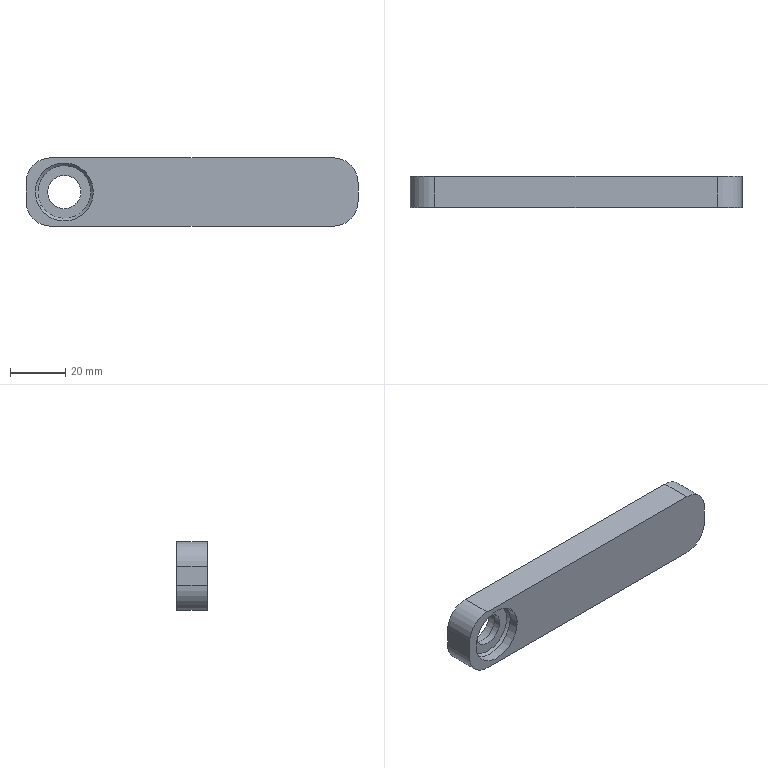Part | NX | 1 solid | 21 faces | box 120 x 11.2 x 24.73 mm | volume 29940 mm3 | cylinder 10 | plane 7 | cone 4 | commonest cylinder face diameters 18 x4 12 x2 15 x2 21 x2
STEP:
#1=CARTESIAN_POINT('',(5242.278,295.631,-304.869));
#2=VERTEX_POINT('',#1);
#3=CARTESIAN_POINT('',(5229.288,295.631,-312.369));
#4=VERTEX_POINT('',#3);
#5=CARTESIAN_POINT('',(5235.783,295.631,-308.619));
#6=DIRECTION('',(0.,-1.,0.));
#7=DIRECTION('',(0.,0.,-1.));
#8=AXIS2_PLACEMENT_3D('',#5,#6,#7);
#9=CIRCLE('',#8,7.5);
#10=EDGE_CURVE('',#2,#4,#9,.T.);
#11=ORIENTED_EDGE('',*,*,#10,.T.);
#12=CARTESIAN_POINT('',(5235.783,295.631,-308.619));
#13=DIRECTION('',(0.,-1.,0.));
#14=DIRECTION('',(0.,0.,-1.));
#15=AXIS2_PLACEMENT_3D('',#12,#13,#14);
#16=CIRCLE('',#15,7.5);
#17=EDGE_CURVE('',#4,#2,#16,.T.);
#18=ORIENTED_EDGE('',*,*,#17,.T.);
#19=EDGE_LOOP('',(#11,#18));
#20=FACE_BOUND('',#19,.T.);
#21=CARTESIAN_POINT('',(5221.929,295.631,-305.254));
#22=VERTEX_POINT('',#21);
#23=CARTESIAN_POINT('',(5221.929,295.631,-311.984));
#24=VERTEX_POINT('',#23);
#25=CARTESIAN_POINT('',(5221.929,295.631,-320.984));
#26=DIRECTION('',(0.,0.,-1.));
#27=VECTOR('',#26,1.);
#28=LINE('',#25,#27);
#29=EDGE_CURVE('',#22,#24,#28,.T.);
#30=ORIENTED_EDGE('',*,*,#29,.F.);
#31=CARTESIAN_POINT('',(5230.929,295.631,-296.254));
#32=VERTEX_POINT('',#31);
#33=CARTESIAN_POINT('',(5230.929,295.631,-305.254));
#34=DIRECTION('',(0.,1.,0.));
#35=DIRECTION('',(0.,0.,-1.));
#36=AXIS2_PLACEMENT_3D('',#33,#34,#35);
#37=CIRCLE('',#36,9.);
#38=EDGE_CURVE('',#22,#32,#37,.T.);
#39=ORIENTED_EDGE('',*,*,#38,.T.);
#40=CARTESIAN_POINT('',(5332.929,295.631,-296.254));
#41=VERTEX_POINT('',#40);
#42=CARTESIAN_POINT('',(5221.929,295.631,-296.254));
#43=DIRECTION('',(-1.,0.,0.));
#44=VECTOR('',#43,1.);
#45=LINE('',#42,#44);
#46=EDGE_CURVE('',#41,#32,#45,.T.);
#47=ORIENTED_EDGE('',*,*,#46,.F.);
#48=CARTESIAN_POINT('',(5341.929,295.631,-305.254));
#49=VERTEX_POINT('',#48);
#50=CARTESIAN_POINT('',(5332.929,295.631,-305.254));
#51=DIRECTION('',(0.,1.,0.));
#52=DIRECTION('',(0.,0.,-1.));
#53=AXIS2_PLACEMENT_3D('',#50,#51,#52);
#54=CIRCLE('',#53,9.);
#55=EDGE_CURVE('',#41,#49,#54,.T.);
#56=ORIENTED_EDGE('',*,*,#55,.T.);
#57=CARTESIAN_POINT('',(5341.929,295.631,-311.984));
#58=VERTEX_POINT('',#57);
#59=CARTESIAN_POINT('',(5341.929,295.631,-296.254));
#60=DIRECTION('',(0.,0.,1.));
#61=VECTOR('',#60,1.);
#62=LINE('',#59,#61);
#63=EDGE_CURVE('',#58,#49,#62,.T.);
#64=ORIENTED_EDGE('',*,*,#63,.F.);
#65=CARTESIAN_POINT('',(5332.929,295.631,-320.984));
#66=VERTEX_POINT('',#65);
#67=CARTESIAN_POINT('',(5332.929,295.631,-311.984));
#68=DIRECTION('',(0.,1.,0.));
#69=DIRECTION('',(0.,0.,-1.));
#70=AXIS2_PLACEMENT_3D('',#67,#68,#69);
#71=CIRCLE('',#70,9.);
#72=EDGE_CURVE('',#58,#66,#71,.T.);
#73=ORIENTED_EDGE('',*,*,#72,.T.);
#74=CARTESIAN_POINT('',(5230.929,295.631,-320.984));
#75=VERTEX_POINT('',#74);
#76=CARTESIAN_POINT('',(5341.929,295.631,-320.984));
#77=DIRECTION('',(1.,0.,0.));
#78=VECTOR('',#77,1.);
#79=LINE('',#76,#78);
#80=EDGE_CURVE('',#75,#66,#79,.T.);
#81=ORIENTED_EDGE('',*,*,#80,.F.);
#82=CARTESIAN_POINT('',(5230.929,295.631,-311.984));
#83=DIRECTION('',(0.,1.,0.));
#84=DIRECTION('',(0.,0.,-1.));
#85=AXIS2_PLACEMENT_3D('',#82,#83,#84);
#86=CIRCLE('',#85,9.);
#87=EDGE_CURVE('',#75,#24,#86,.T.);
#88=ORIENTED_EDGE('',*,*,#87,.T.);
#89=EDGE_LOOP('',(#30,#39,#47,#56,#64,#73,#81,#88));
#90=FACE_BOUND('',#89,.T.);
#91=CARTESIAN_POINT('',(5281.929,295.631,-308.619));
#92=DIRECTION('',(0.,-1.,0.));
#93=DIRECTION('',(-1.,0.,0.));
#94=AXIS2_PLACEMENT_3D('',#91,#92,#93);
#95=PLANE('',#94);
#96=ADVANCED_FACE('',(#20,#90),#95,.F.);
#97=CARTESIAN_POINT('',(5341.929,284.431,-305.254));
#98=VERTEX_POINT('',#97);
#99=CARTESIAN_POINT('',(5341.929,284.431,-311.984));
#100=VERTEX_POINT('',#99);
#101=CARTESIAN_POINT('',(5341.929,284.431,-296.254));
#102=DIRECTION('',(0.,0.,-1.));
#103=VECTOR('',#102,1.);
#104=LINE('',#101,#103);
#105=EDGE_CURVE('',#98,#100,#104,.T.);
#106=ORIENTED_EDGE('',*,*,#105,.T.);
#107=CARTESIAN_POINT('',(5341.929,395.311,-311.984));
#108=DIRECTION('',(0.,1.,0.));
#109=VECTOR('',#108,1.);
#110=LINE('',#107,#109);
#111=EDGE_CURVE('',#100,#58,#110,.T.);
#112=ORIENTED_EDGE('',*,*,#111,.T.);
#113=ORIENTED_EDGE('',*,*,#63,.T.);
#114=CARTESIAN_POINT('',(5341.929,395.311,-305.254));
#115=DIRECTION('',(0.,-1.,0.));
#116=VECTOR('',#115,1.);
#117=LINE('',#114,#116);
#118=EDGE_CURVE('',#49,#98,#117,.T.);
#119=ORIENTED_EDGE('',*,*,#118,.T.);
#120=EDGE_LOOP('',(#106,#112,#113,#119));
#121=FACE_OUTER_BOUND('',#120,.T.);
#122=CARTESIAN_POINT('',(5341.929,395.311,-296.254));
#123=DIRECTION('',(-1.,0.,0.));
#124=DIRECTION('',(0.,0.,1.));
#125=AXIS2_PLACEMENT_3D('',#122,#123,#124);
#126=PLANE('',#125);
#127=ADVANCED_FACE('',(#121),#126,.F.);
#128=CARTESIAN_POINT('',(5226.69,284.431,-313.869));
#129=VERTEX_POINT('',#128);
#130=CARTESIAN_POINT('',(5244.877,284.431,-303.369));
#131=VERTEX_POINT('',#130);
#132=CARTESIAN_POINT('',(5235.783,284.431,-308.619));
#133=DIRECTION('',(0.,1.,0.));
#134=DIRECTION('',(0.,0.,1.));
#135=AXIS2_PLACEMENT_3D('',#132,#133,#134);
#136=CIRCLE('',#135,10.5);
#137=EDGE_CURVE('',#129,#131,#136,.T.);
#138=ORIENTED_EDGE('',*,*,#137,.T.);
#139=CARTESIAN_POINT('',(5235.783,284.431,-308.619));
#140=DIRECTION('',(0.,1.,0.));
#141=DIRECTION('',(0.,0.,1.));
#142=AXIS2_PLACEMENT_3D('',#139,#140,#141);
#143=CIRCLE('',#142,10.5);
#144=EDGE_CURVE('',#131,#129,#143,.T.);
#145=ORIENTED_EDGE('',*,*,#144,.T.);
#146=EDGE_LOOP('',(#138,#145));
#147=FACE_BOUND('',#146,.T.);
#148=CARTESIAN_POINT('',(5230.929,284.431,-296.254));
#149=VERTEX_POINT('',#148);
#150=CARTESIAN_POINT('',(5332.929,284.431,-296.254));
#151=VERTEX_POINT('',#150);
#152=CARTESIAN_POINT('',(5221.929,284.431,-296.254));
#153=DIRECTION('',(1.,0.,0.));
#154=VECTOR('',#153,1.);
#155=LINE('',#152,#154);
#156=EDGE_CURVE('',#149,#151,#155,.T.);
#157=ORIENTED_EDGE('',*,*,#156,.F.);
#158=CARTESIAN_POINT('',(5221.929,284.431,-305.254));
#159=VERTEX_POINT('',#158);
#160=CARTESIAN_POINT('',(5230.929,284.431,-305.254));
#161=DIRECTION('',(0.,-1.,0.));
#162=DIRECTION('',(0.,0.,1.));
#163=AXIS2_PLACEMENT_3D('',#160,#161,#162);
#164=CIRCLE('',#163,9.);
#165=EDGE_CURVE('',#149,#159,#164,.T.);
#166=ORIENTED_EDGE('',*,*,#165,.T.);
#167=CARTESIAN_POINT('',(5221.929,284.431,-311.984));
#168=VERTEX_POINT('',#167);
#169=CARTESIAN_POINT('',(5221.929,284.431,-320.984));
#170=DIRECTION('',(0.,0.,1.));
#171=VECTOR('',#170,1.);
#172=LINE('',#169,#171);
#173=EDGE_CURVE('',#168,#159,#172,.T.);
#174=ORIENTED_EDGE('',*,*,#173,.F.);
#175=CARTESIAN_POINT('',(5230.929,284.431,-320.984));
#176=VERTEX_POINT('',#175);
#177=CARTESIAN_POINT('',(5230.929,284.431,-311.984));
#178=DIRECTION('',(0.,-1.,0.));
#179=DIRECTION('',(0.,0.,1.));
#180=AXIS2_PLACEMENT_3D('',#177,#178,#179);
#181=CIRCLE('',#180,9.);
#182=EDGE_CURVE('',#168,#176,#181,.T.);
#183=ORIENTED_EDGE('',*,*,#182,.T.);
#184=CARTESIAN_POINT('',(5332.929,284.431,-320.984));
#185=VERTEX_POINT('',#184);
#186=CARTESIAN_POINT('',(5341.929,284.431,-320.984));
#187=DIRECTION('',(-1.,0.,0.));
#188=VECTOR('',#187,1.);
#189=LINE('',#186,#188);
#190=EDGE_CURVE('',#185,#176,#189,.T.);
#191=ORIENTED_EDGE('',*,*,#190,.F.);
#192=CARTESIAN_POINT('',(5332.929,284.431,-311.984));
#193=DIRECTION('',(0.,-1.,0.));
#194=DIRECTION('',(0.,0.,1.));
#195=AXIS2_PLACEMENT_3D('',#192,#193,#194);
#196=CIRCLE('',#195,9.);
#197=EDGE_CURVE('',#185,#100,#196,.T.);
#198=ORIENTED_EDGE('',*,*,#197,.T.);
#199=ORIENTED_EDGE('',*,*,#105,.F.);
#200=CARTESIAN_POINT('',(5332.929,284.431,-305.254));
#201=DIRECTION('',(0.,-1.,0.));
#202=DIRECTION('',(0.,0.,1.));
#203=AXIS2_PLACEMENT_3D('',#200,#201,#202);
#204=CIRCLE('',#203,9.);
#205=EDGE_CURVE('',#98,#151,#204,.T.);
#206=ORIENTED_EDGE('',*,*,#205,.T.);
#207=EDGE_LOOP('',(#157,#166,#174,#183,#191,#198,#199,#206));
#208=FACE_BOUND('',#207,.T.);
#209=CARTESIAN_POINT('',(0.,284.431,0.));
#210=DIRECTION('',(0.,1.,0.));
#211=DIRECTION('',(0.,0.,1.));
#212=AXIS2_PLACEMENT_3D('',#209,#210,#211);
#213=PLANE('',#212);
#214=ADVANCED_FACE('',(#147,#208),#213,.F.);
#215=ORIENTED_EDGE('',*,*,#190,.T.);
#216=CARTESIAN_POINT('',(5230.929,395.311,-320.984));
#217=DIRECTION('',(0.,1.,0.));
#218=VECTOR('',#217,1.);
#219=LINE('',#216,#218);
#220=EDGE_CURVE('',#176,#75,#219,.T.);
#221=ORIENTED_EDGE('',*,*,#220,.T.);
#222=ORIENTED_EDGE('',*,*,#80,.T.);
#223=CARTESIAN_POINT('',(5332.929,395.311,-320.984));
#224=DIRECTION('',(0.,-1.,0.));
#225=VECTOR('',#224,1.);
#226=LINE('',#223,#225);
#227=EDGE_CURVE('',#66,#185,#226,.T.);
#228=ORIENTED_EDGE('',*,*,#227,.T.);
#229=EDGE_LOOP('',(#215,#221,#222,#228));
#230=FACE_OUTER_BOUND('',#229,.T.);
#231=CARTESIAN_POINT('',(5341.929,395.311,-320.984));
#232=DIRECTION('',(0.,0.,1.));
#233=DIRECTION('',(1.,0.,0.));
#234=AXIS2_PLACEMENT_3D('',#231,#232,#233);
#235=PLANE('',#234);
#236=ADVANCED_FACE('',(#230),#235,.F.);
#237=ORIENTED_EDGE('',*,*,#46,.T.);
#238=CARTESIAN_POINT('',(5230.929,395.311,-296.254));
#239=DIRECTION('',(0.,-1.,0.));
#240=VECTOR('',#239,1.);
#241=LINE('',#238,#240);
#242=EDGE_CURVE('',#32,#149,#241,.T.);
#243=ORIENTED_EDGE('',*,*,#242,.T.);
#244=ORIENTED_EDGE('',*,*,#156,.T.);
#245=CARTESIAN_POINT('',(5332.929,395.311,-296.254));
#246=DIRECTION('',(0.,1.,0.));
#247=VECTOR('',#246,1.);
#248=LINE('',#245,#247);
#249=EDGE_CURVE('',#151,#41,#248,.T.);
#250=ORIENTED_EDGE('',*,*,#249,.T.);
#251=EDGE_LOOP('',(#237,#243,#244,#250));
#252=FACE_OUTER_BOUND('',#251,.T.);
#253=CARTESIAN_POINT('',(5221.929,395.311,-296.254));
#254=DIRECTION('',(0.,0.,-1.));
#255=DIRECTION('',(-1.,0.,0.));
#256=AXIS2_PLACEMENT_3D('',#253,#254,#255);
#257=PLANE('',#256);
#258=ADVANCED_FACE('',(#252),#257,.F.);
#259=ORIENTED_EDGE('',*,*,#173,.T.);
#260=CARTESIAN_POINT('',(5221.929,395.311,-305.254));
#261=DIRECTION('',(0.,1.,0.));
#262=VECTOR('',#261,1.);
#263=LINE('',#260,#262);
#264=EDGE_CURVE('',#159,#22,#263,.T.);
#265=ORIENTED_EDGE('',*,*,#264,.T.);
#266=ORIENTED_EDGE('',*,*,#29,.T.);
#267=CARTESIAN_POINT('',(5221.929,395.311,-311.984));
#268=DIRECTION('',(0.,-1.,0.));
#269=VECTOR('',#268,1.);
#270=LINE('',#267,#269);
#271=EDGE_CURVE('',#24,#168,#270,.T.);
#272=ORIENTED_EDGE('',*,*,#271,.T.);
#273=EDGE_LOOP('',(#259,#265,#266,#272));
#274=FACE_OUTER_BOUND('',#273,.T.);
#275=CARTESIAN_POINT('',(5221.929,395.311,-320.984));
#276=DIRECTION('',(1.,0.,0.));
#277=DIRECTION('',(0.,0.,-1.));
#278=AXIS2_PLACEMENT_3D('',#275,#276,#277);
#279=PLANE('',#278);
#280=ADVANCED_FACE('',(#274),#279,.F.);
#281=ORIENTED_EDGE('',*,*,#38,.F.);
#282=ORIENTED_EDGE('',*,*,#264,.F.);
#283=ORIENTED_EDGE('',*,*,#165,.F.);
#284=ORIENTED_EDGE('',*,*,#242,.F.);
#285=EDGE_LOOP('',(#281,#282,#283,#284));
#286=FACE_OUTER_BOUND('',#285,.T.);
#287=CARTESIAN_POINT('',(5230.929,395.311,-305.254));
#288=DIRECTION('',(0.,-1.,0.));
#289=DIRECTION('',(0.,0.,-1.));
#290=AXIS2_PLACEMENT_3D('',#287,#288,#289);
#291=CYLINDRICAL_SURFACE('',#290,9.);
#292=ADVANCED_FACE('',(#286),#291,.T.);
#293=ORIENTED_EDGE('',*,*,#87,.F.);
#294=ORIENTED_EDGE('',*,*,#220,.F.);
#295=ORIENTED_EDGE('',*,*,#182,.F.);
#296=ORIENTED_EDGE('',*,*,#271,.F.);
#297=EDGE_LOOP('',(#293,#294,#295,#296));
#298=FACE_OUTER_BOUND('',#297,.T.);
#299=CARTESIAN_POINT('',(5230.929,395.311,-311.984));
#300=DIRECTION('',(0.,-1.,0.));
#301=DIRECTION('',(0.,0.,-1.));
#302=AXIS2_PLACEMENT_3D('',#299,#300,#301);
#303=CYLINDRICAL_SURFACE('',#302,9.);
#304=ADVANCED_FACE('',(#298),#303,.T.);
#305=ORIENTED_EDGE('',*,*,#72,.F.);
#306=ORIENTED_EDGE('',*,*,#111,.F.);
#307=ORIENTED_EDGE('',*,*,#197,.F.);
#308=ORIENTED_EDGE('',*,*,#227,.F.);
#309=EDGE_LOOP('',(#305,#306,#307,#308));
#310=FACE_OUTER_BOUND('',#309,.T.);
#311=CARTESIAN_POINT('',(5332.929,395.311,-311.984));
#312=DIRECTION('',(0.,-1.,0.));
#313=DIRECTION('',(0.,0.,-1.));
#314=AXIS2_PLACEMENT_3D('',#311,#312,#313);
#315=CYLINDRICAL_SURFACE('',#314,9.);
#316=ADVANCED_FACE('',(#310),#315,.T.);
#317=ORIENTED_EDGE('',*,*,#55,.F.);
#318=ORIENTED_EDGE('',*,*,#249,.F.);
#319=ORIENTED_EDGE('',*,*,#205,.F.);
#320=ORIENTED_EDGE('',*,*,#118,.F.);
#321=EDGE_LOOP('',(#317,#318,#319,#320));
#322=FACE_OUTER_BOUND('',#321,.T.);
#323=CARTESIAN_POINT('',(5332.929,395.311,-305.254));
#324=DIRECTION('',(0.,-1.,0.));
#325=DIRECTION('',(0.,0.,-1.));
#326=AXIS2_PLACEMENT_3D('',#323,#324,#325);
#327=CYLINDRICAL_SURFACE('',#326,9.);
#328=ADVANCED_FACE('',(#322),#327,.T.);
#329=CARTESIAN_POINT('',(5240.979,291.48,-305.619));
#330=VERTEX_POINT('',#329);
#331=CARTESIAN_POINT('',(5230.587,291.48,-311.619));
#332=VERTEX_POINT('',#331);
#333=CARTESIAN_POINT('',(5235.783,291.48,-308.619));
#334=DIRECTION('',(0.,1.,0.));
#335=DIRECTION('',(-0.866,0.,-0.5));
#336=AXIS2_PLACEMENT_3D('',#333,#334,#335);
#337=CIRCLE('',#336,6.);
#338=EDGE_CURVE('',#330,#332,#337,.T.);
#339=ORIENTED_EDGE('',*,*,#338,.T.);
#340=CARTESIAN_POINT('',(5230.587,288.931,-311.619));
#341=VERTEX_POINT('',#340);
#342=CARTESIAN_POINT('',(5230.587,291.931,-311.619));
#343=DIRECTION('',(0.,1.,0.));
#344=VECTOR('',#343,1.);
#345=LINE('',#342,#344);
#346=EDGE_CURVE('',#341,#332,#345,.T.);
#347=ORIENTED_EDGE('',*,*,#346,.F.);
#348=CARTESIAN_POINT('',(5240.979,288.931,-305.619));
#349=VERTEX_POINT('',#348);
#350=CARTESIAN_POINT('',(5235.783,288.931,-308.619));
#351=DIRECTION('',(0.,1.,0.));
#352=DIRECTION('',(-0.866,0.,-0.5));
#353=AXIS2_PLACEMENT_3D('',#350,#351,#352);
#354=CIRCLE('',#353,6.);
#355=EDGE_CURVE('',#349,#341,#354,.T.);
#356=ORIENTED_EDGE('',*,*,#355,.F.);
#357=CARTESIAN_POINT('',(5240.979,291.931,-305.619));
#358=DIRECTION('',(0.,-1.,0.));
#359=VECTOR('',#358,1.);
#360=LINE('',#357,#359);
#361=EDGE_CURVE('',#330,#349,#360,.T.);
#362=ORIENTED_EDGE('',*,*,#361,.F.);
#363=EDGE_LOOP('',(#339,#347,#356,#362));
#364=FACE_OUTER_BOUND('',#363,.T.);
#365=CARTESIAN_POINT('',(5235.783,291.931,-308.619));
#366=DIRECTION('',(0.,-1.,0.));
#367=DIRECTION('',(0.866,0.,0.5));
#368=AXIS2_PLACEMENT_3D('',#365,#366,#367);
#369=CYLINDRICAL_SURFACE('',#368,6.);
#370=ADVANCED_FACE('',(#364),#369,.F.);
#371=CARTESIAN_POINT('',(5244.08,288.931,-303.829));
#372=VERTEX_POINT('',#371);
#373=CARTESIAN_POINT('',(5227.487,288.931,-313.409));
#374=VERTEX_POINT('',#373);
#375=CARTESIAN_POINT('',(5235.783,288.931,-308.619));
#376=DIRECTION('',(0.,1.,0.));
#377=DIRECTION('',(-0.866,0.,-0.5));
#378=AXIS2_PLACEMENT_3D('',#375,#376,#377);
#379=CIRCLE('',#378,9.58);
#380=EDGE_CURVE('',#372,#374,#379,.T.);
#381=ORIENTED_EDGE('',*,*,#380,.F.);
#382=CARTESIAN_POINT('',(5235.783,288.931,-308.619));
#383=DIRECTION('',(0.,1.,0.));
#384=DIRECTION('',(-0.866,0.,-0.5));
#385=AXIS2_PLACEMENT_3D('',#382,#383,#384);
#386=CIRCLE('',#385,9.58);
#387=EDGE_CURVE('',#374,#372,#386,.T.);
#388=ORIENTED_EDGE('',*,*,#387,.F.);
#389=EDGE_LOOP('',(#381,#388));
#390=FACE_BOUND('',#389,.T.);
#391=ORIENTED_EDGE('',*,*,#355,.T.);
#392=CARTESIAN_POINT('',(5235.783,288.931,-308.619));
#393=DIRECTION('',(0.,1.,0.));
#394=DIRECTION('',(-0.866,0.,-0.5));
#395=AXIS2_PLACEMENT_3D('',#392,#393,#394);
#396=CIRCLE('',#395,6.);
#397=EDGE_CURVE('',#341,#349,#396,.T.);
#398=ORIENTED_EDGE('',*,*,#397,.T.);
#399=EDGE_LOOP('',(#391,#398));
#400=FACE_BOUND('',#399,.T.);
#401=CARTESIAN_POINT('',(5244.08,288.931,-303.829));
#402=DIRECTION('',(0.,-1.,0.));
#403=DIRECTION('',(0.866,0.,0.5));
#404=AXIS2_PLACEMENT_3D('',#401,#402,#403);
#405=PLANE('',#404);
#406=ADVANCED_FACE('',(#390,#400),#405,.T.);
#407=ORIENTED_EDGE('',*,*,#380,.T.);
#408=CARTESIAN_POINT('',(5226.69,288.01,-313.869));
#409=VERTEX_POINT('',#408);
#410=CARTESIAN_POINT('',(5227.487,288.931,-313.409));
#411=DIRECTION('',(0.6124,0.7071,0.3536));
#412=VECTOR('',#411,1.);
#413=LINE('',#410,#412);
#414=EDGE_CURVE('',#409,#374,#413,.T.);
#415=ORIENTED_EDGE('',*,*,#414,.F.);
#416=CARTESIAN_POINT('',(5244.877,288.01,-303.369));
#417=VERTEX_POINT('',#416);
#418=CARTESIAN_POINT('',(5235.783,288.01,-308.619));
#419=DIRECTION('',(0.,1.,0.));
#420=DIRECTION('',(-0.866,0.,-0.5));
#421=AXIS2_PLACEMENT_3D('',#418,#419,#420);
#422=CIRCLE('',#421,10.5);
#423=EDGE_CURVE('',#417,#409,#422,.T.);
#424=ORIENTED_EDGE('',*,*,#423,.F.);
#425=CARTESIAN_POINT('',(5244.08,288.931,-303.829));
#426=DIRECTION('',(0.6124,-0.7071,0.3536));
#427=VECTOR('',#426,1.);
#428=LINE('',#425,#427);
#429=EDGE_CURVE('',#372,#417,#428,.T.);
#430=ORIENTED_EDGE('',*,*,#429,.F.);
#431=EDGE_LOOP('',(#407,#415,#424,#430));
#432=FACE_OUTER_BOUND('',#431,.T.);
#433=CARTESIAN_POINT('',(5235.783,288.931,-308.619));
#434=DIRECTION('',(0.,-1.,0.));
#435=DIRECTION('',(0.866,0.,0.5));
#436=AXIS2_PLACEMENT_3D('',#433,#434,#435);
#437=CONICAL_SURFACE('',#436,9.58,45.);
#438=ADVANCED_FACE('',(#432),#437,.F.);
#439=ORIENTED_EDGE('',*,*,#429,.T.);
#440=CARTESIAN_POINT('',(5235.783,288.01,-308.619));
#441=DIRECTION('',(0.,1.,0.));
#442=DIRECTION('',(-0.866,0.,-0.5));
#443=AXIS2_PLACEMENT_3D('',#440,#441,#442);
#444=CIRCLE('',#443,10.5);
#445=EDGE_CURVE('',#409,#417,#444,.T.);
#446=ORIENTED_EDGE('',*,*,#445,.F.);
#447=ORIENTED_EDGE('',*,*,#414,.T.);
#448=ORIENTED_EDGE('',*,*,#387,.T.);
#449=EDGE_LOOP('',(#439,#446,#447,#448));
#450=FACE_OUTER_BOUND('',#449,.T.);
#451=CARTESIAN_POINT('',(5235.783,288.931,-308.619));
#452=DIRECTION('',(0.,-1.,0.));
#453=DIRECTION('',(0.866,0.,0.5));
#454=AXIS2_PLACEMENT_3D('',#451,#452,#453);
#455=CONICAL_SURFACE('',#454,9.58,45.);
#456=ADVANCED_FACE('',(#450),#455,.F.);
#457=CARTESIAN_POINT('',(5226.69,291.931,-313.869));
#458=DIRECTION('',(0.,1.,0.));
#459=VECTOR('',#458,1.);
#460=LINE('',#457,#459);
#461=EDGE_CURVE('',#129,#409,#460,.T.);
#462=ORIENTED_EDGE('',*,*,#461,.T.);
#463=ORIENTED_EDGE('',*,*,#445,.T.);
#464=CARTESIAN_POINT('',(5244.877,291.931,-303.369));
#465=DIRECTION('',(0.,-1.,0.));
#466=VECTOR('',#465,1.);
#467=LINE('',#464,#466);
#468=EDGE_CURVE('',#417,#131,#467,.T.);
#469=ORIENTED_EDGE('',*,*,#468,.T.);
#470=ORIENTED_EDGE('',*,*,#137,.F.);
#471=EDGE_LOOP('',(#462,#463,#469,#470));
#472=FACE_OUTER_BOUND('',#471,.T.);
#473=CARTESIAN_POINT('',(5235.783,291.931,-308.619));
#474=DIRECTION('',(0.,-1.,0.));
#475=DIRECTION('',(0.866,0.,0.5));
#476=AXIS2_PLACEMENT_3D('',#473,#474,#475);
#477=CYLINDRICAL_SURFACE('',#476,10.5);
#478=ADVANCED_FACE('',(#472),#477,.F.);
#479=ORIENTED_EDGE('',*,*,#468,.F.);
#480=ORIENTED_EDGE('',*,*,#423,.T.);
#481=ORIENTED_EDGE('',*,*,#461,.F.);
#482=ORIENTED_EDGE('',*,*,#144,.F.);
#483=EDGE_LOOP('',(#479,#480,#481,#482));
#484=FACE_OUTER_BOUND('',#483,.T.);
#485=CARTESIAN_POINT('',(5235.783,291.931,-308.619));
#486=DIRECTION('',(0.,-1.,0.));
#487=DIRECTION('',(0.866,0.,0.5));
#488=AXIS2_PLACEMENT_3D('',#485,#486,#487);
#489=CYLINDRICAL_SURFACE('',#488,10.5);
#490=ADVANCED_FACE('',(#484),#489,.F.);
#491=ORIENTED_EDGE('',*,*,#361,.T.);
#492=ORIENTED_EDGE('',*,*,#397,.F.);
#493=ORIENTED_EDGE('',*,*,#346,.T.);
#494=CARTESIAN_POINT('',(5235.783,291.48,-308.619));
#495=DIRECTION('',(0.,1.,0.));
#496=DIRECTION('',(-0.866,0.,-0.5));
#497=AXIS2_PLACEMENT_3D('',#494,#495,#496);
#498=CIRCLE('',#497,6.);
#499=EDGE_CURVE('',#332,#330,#498,.T.);
#500=ORIENTED_EDGE('',*,*,#499,.T.);
#501=EDGE_LOOP('',(#491,#492,#493,#500));
#502=FACE_OUTER_BOUND('',#501,.T.);
#503=CARTESIAN_POINT('',(5235.783,291.931,-308.619));
#504=DIRECTION('',(0.,-1.,0.));
#505=DIRECTION('',(0.866,0.,0.5));
#506=AXIS2_PLACEMENT_3D('',#503,#504,#505);
#507=CYLINDRICAL_SURFACE('',#506,6.);
#508=ADVANCED_FACE('',(#502),#507,.F.);
#509=ORIENTED_EDGE('',*,*,#338,.F.);
#510=CARTESIAN_POINT('',(5242.278,292.531,-304.869));
#511=VERTEX_POINT('',#510);
#512=CARTESIAN_POINT('',(5242.278,292.531,-304.869));
#513=DIRECTION('',(0.7094,0.5736,0.4096));
#514=VECTOR('',#513,1.);
#515=LINE('',#512,#514);
#516=EDGE_CURVE('',#330,#511,#515,.T.);
#517=ORIENTED_EDGE('',*,*,#516,.T.);
#518=CARTESIAN_POINT('',(5229.288,292.531,-312.369));
#519=VERTEX_POINT('',#518);
#520=CARTESIAN_POINT('',(5235.783,292.531,-308.619));
#521=DIRECTION('',(0.,1.,0.));
#522=DIRECTION('',(-0.866,0.,-0.5));
#523=AXIS2_PLACEMENT_3D('',#520,#521,#522);
#524=CIRCLE('',#523,7.5);
#525=EDGE_CURVE('',#511,#519,#524,.T.);
#526=ORIENTED_EDGE('',*,*,#525,.T.);
#527=CARTESIAN_POINT('',(5229.288,292.531,-312.369));
#528=DIRECTION('',(0.7094,-0.5736,0.4096));
#529=VECTOR('',#528,1.);
#530=LINE('',#527,#529);
#531=EDGE_CURVE('',#519,#332,#530,.T.);
#532=ORIENTED_EDGE('',*,*,#531,.T.);
#533=EDGE_LOOP('',(#509,#517,#526,#532));
#534=FACE_OUTER_BOUND('',#533,.T.);
#535=CARTESIAN_POINT('',(5235.783,292.531,-308.619));
#536=DIRECTION('',(0.,1.,0.));
#537=DIRECTION('',(-0.866,0.,-0.5));
#538=AXIS2_PLACEMENT_3D('',#535,#536,#537);
#539=CONICAL_SURFACE('',#538,7.5,55.);
#540=ADVANCED_FACE('',(#534),#539,.F.);
#541=ORIENTED_EDGE('',*,*,#531,.F.);
#542=CARTESIAN_POINT('',(5235.783,292.531,-308.619));
#543=DIRECTION('',(0.,1.,0.));
#544=DIRECTION('',(-0.866,0.,-0.5));
#545=AXIS2_PLACEMENT_3D('',#542,#543,#544);
#546=CIRCLE('',#545,7.5);
#547=EDGE_CURVE('',#519,#511,#546,.T.);
#548=ORIENTED_EDGE('',*,*,#547,.T.);
#549=ORIENTED_EDGE('',*,*,#516,.F.);
#550=ORIENTED_EDGE('',*,*,#499,.F.);
#551=EDGE_LOOP('',(#541,#548,#549,#550));
#552=FACE_OUTER_BOUND('',#551,.T.);
#553=CARTESIAN_POINT('',(5235.783,292.531,-308.619));
#554=DIRECTION('',(0.,1.,0.));
#555=DIRECTION('',(-0.866,0.,-0.5));
#556=AXIS2_PLACEMENT_3D('',#553,#554,#555);
#557=CONICAL_SURFACE('',#556,7.5,55.);
#558=ADVANCED_FACE('',(#552),#557,.F.);
#559=CARTESIAN_POINT('',(5242.278,291.931,-304.869));
#560=DIRECTION('',(0.,-1.,0.));
#561=VECTOR('',#560,1.);
#562=LINE('',#559,#561);
#563=EDGE_CURVE('',#2,#511,#562,.T.);
#564=ORIENTED_EDGE('',*,*,#563,.T.);
#565=ORIENTED_EDGE('',*,*,#547,.F.);
#566=CARTESIAN_POINT('',(5229.288,291.931,-312.369));
#567=DIRECTION('',(0.,1.,0.));
#568=VECTOR('',#567,1.);
#569=LINE('',#566,#568);
#570=EDGE_CURVE('',#519,#4,#569,.T.);
#571=ORIENTED_EDGE('',*,*,#570,.T.);
#572=ORIENTED_EDGE('',*,*,#10,.F.);
#573=EDGE_LOOP('',(#564,#565,#571,#572));
#574=FACE_OUTER_BOUND('',#573,.T.);
#575=CARTESIAN_POINT('',(5235.783,291.931,-308.619));
#576=DIRECTION('',(0.,-1.,0.));
#577=DIRECTION('',(0.866,0.,0.5));
#578=AXIS2_PLACEMENT_3D('',#575,#576,#577);
#579=CYLINDRICAL_SURFACE('',#578,7.5);
#580=ADVANCED_FACE('',(#574),#579,.F.);
#581=ORIENTED_EDGE('',*,*,#570,.F.);
#582=ORIENTED_EDGE('',*,*,#525,.F.);
#583=ORIENTED_EDGE('',*,*,#563,.F.);
#584=ORIENTED_EDGE('',*,*,#17,.F.);
#585=EDGE_LOOP('',(#581,#582,#583,#584));
#586=FACE_OUTER_BOUND('',#585,.T.);
#587=CARTESIAN_POINT('',(5235.783,291.931,-308.619));
#588=DIRECTION('',(0.,-1.,0.));
#589=DIRECTION('',(0.866,0.,0.5));
#590=AXIS2_PLACEMENT_3D('',#587,#588,#589);
#591=CYLINDRICAL_SURFACE('',#590,7.5);
#592=ADVANCED_FACE('',(#586),#591,.F.);
#593=CLOSED_SHELL('',(#96,#127,#214,#236,#258,#280,#292,#304,#316,#328,#370,#406,#438,#456,#478,#490,#508,#540,#558,#580,#592));
#594=MANIFOLD_SOLID_BREP('',#593);
#595=(LENGTH_UNIT()NAMED_UNIT(*)SI_UNIT(.MILLI.,.METRE.));
#596=UNCERTAINTY_MEASURE_WITH_UNIT(LENGTH_MEASURE(0.00002),#595,'','');
#597=(NAMED_UNIT(*)PLANE_ANGLE_UNIT()SI_UNIT($,.RADIAN.));
#598=PLANE_ANGLE_MEASURE_WITH_UNIT(PLANE_ANGLE_MEASURE(0.01745),#597);
#599=DIMENSIONAL_EXPONENTS(0.,0.,0.,0.,0.,0.,0.);
#600=(CONVERSION_BASED_UNIT('DEGREE',#598)NAMED_UNIT(#599)PLANE_ANGLE_UNIT());
#601=(NAMED_UNIT(*)SI_UNIT($,.STERADIAN.)SOLID_ANGLE_UNIT());
#602=(GEOMETRIC_REPRESENTATION_CONTEXT(3)GLOBAL_UNCERTAINTY_ASSIGNED_CONTEXT((#596))GLOBAL_UNIT_ASSIGNED_CONTEXT((#595,#600,#601))REPRESENTATION_CONTEXT('',''));
#603=ADVANCED_BREP_SHAPE_REPRESENTATION('',(#594),#602);